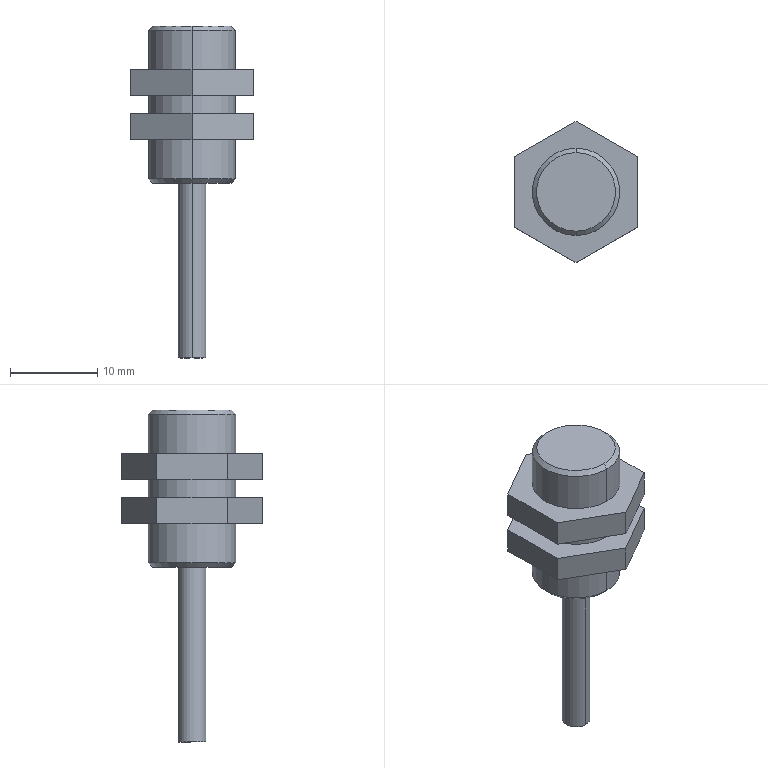Part | STEP file | SceondEH-110 | 3 solids | 31 faces | box 14 x 16.166 x 38 mm | volume 2114 mm3 | plane 19 | cylinder 8 | cone 4 | commonest cylinder face diameters 10 x6 3.2 x2